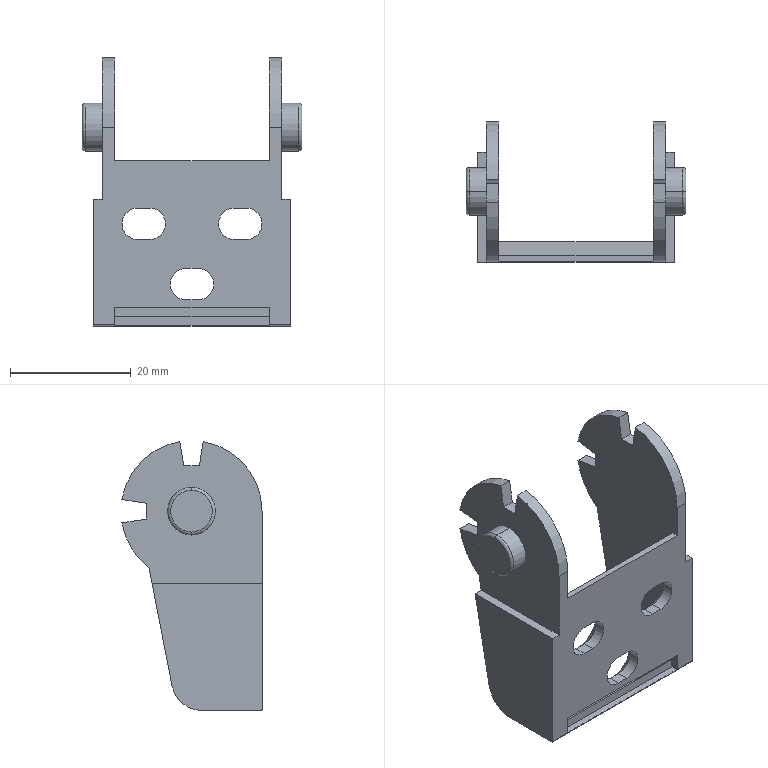Part | 1 solid | 77 faces | box 36.4 x 23.217 x 44.527 mm | volume 6177 mm3 | plane 48 | cylinder 19 | cone 6 | torus 4 | commonest cylinder face diameters 5.2 x6 23.38 x6 7.9 x4 10.1 x2 0.5 x1